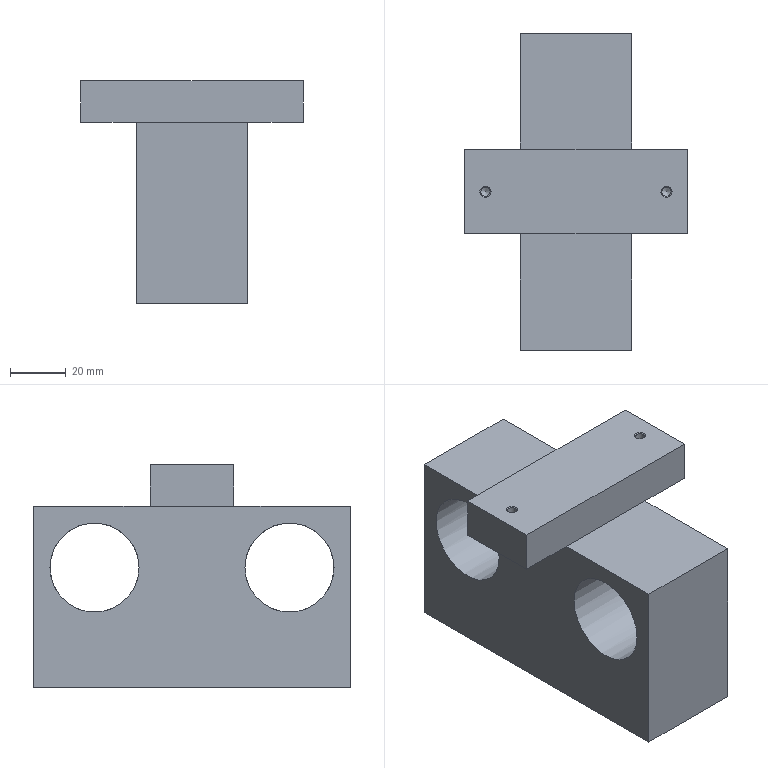Part | STEP file | Tube feed_id350_x_t | 1 solid | 22 faces | box 80 x 114 x 80 mm | volume 267916 mm3 | plane 14 | cylinder 4 | cone 4 | commonest cylinder face diameters 3.3 x2 32 x2